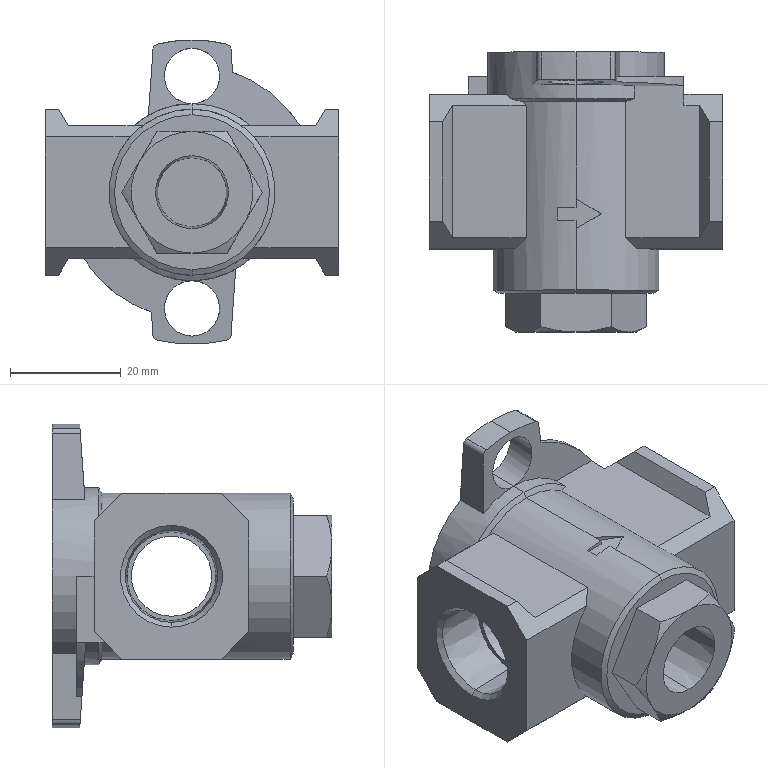Part | STEP file | VHS30-03_VHS3035BA Body_30 | 1 solid | 109 faces | box 53 x 50.6 x 55 mm | volume 43181 mm3 | plane 66 | cylinder 22 | cone 21 | commonest cylinder face diameters 2 x4 10 x4 14.5 x4 32 x3 55 x3 30 x2